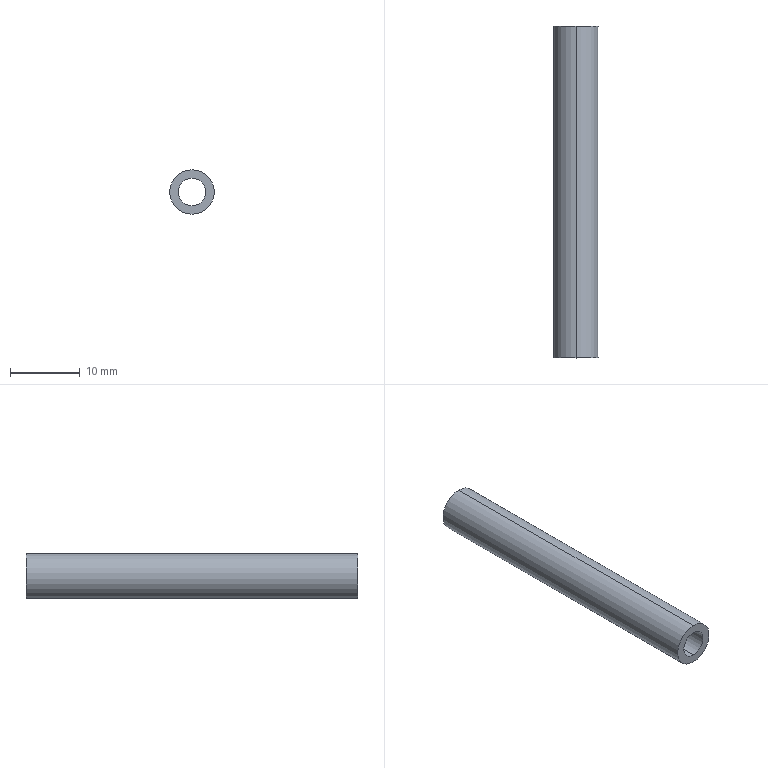Part | NX | features BREP 1 | 1 solid | 6 faces | box 6.35 x 47.5 x 6.35 mm | volume 933.944 mm3 | cylinder 4 | plane 2 | commonest cylinder face diameters 3.91 x2 6.35 x2
STEP:
#1=CARTESIAN_POINT('',(0.,376.,1.955));
#2=VERTEX_POINT('',#1);
#3=CARTESIAN_POINT('',(0.,328.5,1.955));
#4=VERTEX_POINT('',#3);
#5=CARTESIAN_POINT('',(0.,328.5,1.955));
#6=DIRECTION('',(0.,1.,0.));
#7=VECTOR('',#6,1000.);
#8=LINE('',#5,#7);
#9=EDGE_CURVE('',#2,#4,#8,.F.);
#10=ORIENTED_EDGE('',*,*,#9,.T.);
#11=CARTESIAN_POINT('',(0.,328.5,-1.955));
#12=VERTEX_POINT('',#11);
#13=CARTESIAN_POINT('',(0.,328.5,0.));
#14=DIRECTION('',(0.,1.,0.));
#15=DIRECTION('',(-1.,0.,0.));
#16=AXIS2_PLACEMENT_3D('',#13,#14,#15);
#17=CIRCLE('',#16,1.955);
#18=EDGE_CURVE('',#12,#4,#17,.T.);
#19=ORIENTED_EDGE('',*,*,#18,.F.);
#20=CARTESIAN_POINT('',(0.,376.,-1.955));
#21=VERTEX_POINT('',#20);
#22=CARTESIAN_POINT('',(0.,328.5,-1.955));
#23=DIRECTION('',(0.,1.,0.));
#24=VECTOR('',#23,1000.);
#25=LINE('',#22,#24);
#26=EDGE_CURVE('',#21,#12,#25,.F.);
#27=ORIENTED_EDGE('',*,*,#26,.F.);
#28=CARTESIAN_POINT('',(0.,376.,0.));
#29=DIRECTION('',(0.,-1.,0.));
#30=DIRECTION('',(0.,0.,1.));
#31=AXIS2_PLACEMENT_3D('',#28,#29,#30);
#32=CIRCLE('',#31,1.955);
#33=EDGE_CURVE('',#2,#21,#32,.T.);
#34=ORIENTED_EDGE('',*,*,#33,.F.);
#35=EDGE_LOOP('',(#10,#19,#27,#34));
#36=FACE_BOUND('',#35,.T.);
#37=CARTESIAN_POINT('',(0.,376.,0.));
#38=DIRECTION('',(0.,-1.,0.));
#39=DIRECTION('',(0.,0.,-1.));
#40=AXIS2_PLACEMENT_3D('',#37,#38,#39);
#41=CYLINDRICAL_SURFACE('',#40,1.955);
#42=ADVANCED_FACE('',(#36),#41,.F.);
#43=CARTESIAN_POINT('',(0.,376.,-3.175));
#44=VERTEX_POINT('',#43);
#45=CARTESIAN_POINT('',(0.,376.,3.175));
#46=VERTEX_POINT('',#45);
#47=CARTESIAN_POINT('',(0.,376.,0.));
#48=DIRECTION('',(0.,1.,0.));
#49=DIRECTION('',(-1.,0.,0.));
#50=AXIS2_PLACEMENT_3D('',#47,#48,#49);
#51=CIRCLE('',#50,3.175);
#52=EDGE_CURVE('',#44,#46,#51,.T.);
#53=ORIENTED_EDGE('',*,*,#52,.T.);
#54=CARTESIAN_POINT('',(0.,376.,0.));
#55=DIRECTION('',(0.,1.,0.));
#56=DIRECTION('',(0.,0.,1.));
#57=AXIS2_PLACEMENT_3D('',#54,#55,#56);
#58=CIRCLE('',#57,3.175);
#59=EDGE_CURVE('',#46,#44,#58,.T.);
#60=ORIENTED_EDGE('',*,*,#59,.T.);
#61=EDGE_LOOP('',(#53,#60));
#62=FACE_BOUND('',#61,.T.);
#63=CARTESIAN_POINT('',(0.,376.,0.));
#64=DIRECTION('',(0.,-1.,0.));
#65=DIRECTION('',(0.,0.,-1.));
#66=AXIS2_PLACEMENT_3D('',#63,#64,#65);
#67=CIRCLE('',#66,1.955);
#68=EDGE_CURVE('',#21,#2,#67,.T.);
#69=ORIENTED_EDGE('',*,*,#68,.T.);
#70=ORIENTED_EDGE('',*,*,#33,.T.);
#71=EDGE_LOOP('',(#69,#70));
#72=FACE_BOUND('',#71,.T.);
#73=CARTESIAN_POINT('',(0.,376.,0.));
#74=DIRECTION('',(0.,1.,0.));
#75=DIRECTION('',(1.,0.,0.));
#76=AXIS2_PLACEMENT_3D('',#73,#74,#75);
#77=PLANE('',#76);
#78=ADVANCED_FACE('',(#62,#72),#77,.T.);
#79=ORIENTED_EDGE('',*,*,#52,.F.);
#80=CARTESIAN_POINT('',(0.,328.5,-3.175));
#81=VERTEX_POINT('',#80);
#82=CARTESIAN_POINT('',(0.,328.5,-3.175));
#83=DIRECTION('',(0.,1.,0.));
#84=VECTOR('',#83,1000.);
#85=LINE('',#82,#84);
#86=EDGE_CURVE('',#81,#44,#85,.T.);
#87=ORIENTED_EDGE('',*,*,#86,.F.);
#88=CARTESIAN_POINT('',(0.,328.5,3.175));
#89=VERTEX_POINT('',#88);
#90=CARTESIAN_POINT('',(0.,328.5,0.));
#91=DIRECTION('',(0.,-1.,0.));
#92=DIRECTION('',(0.,0.,1.));
#93=AXIS2_PLACEMENT_3D('',#90,#91,#92);
#94=CIRCLE('',#93,3.175);
#95=EDGE_CURVE('',#89,#81,#94,.T.);
#96=ORIENTED_EDGE('',*,*,#95,.F.);
#97=CARTESIAN_POINT('',(0.,328.5,3.175));
#98=DIRECTION('',(0.,1.,0.));
#99=VECTOR('',#98,1000.);
#100=LINE('',#97,#99);
#101=EDGE_CURVE('',#89,#46,#100,.T.);
#102=ORIENTED_EDGE('',*,*,#101,.T.);
#103=EDGE_LOOP('',(#79,#87,#96,#102));
#104=FACE_BOUND('',#103,.T.);
#105=CARTESIAN_POINT('',(0.,376.,0.));
#106=DIRECTION('',(0.,-1.,0.));
#107=DIRECTION('',(0.,0.,-1.));
#108=AXIS2_PLACEMENT_3D('',#105,#106,#107);
#109=CYLINDRICAL_SURFACE('',#108,3.175);
#110=ADVANCED_FACE('',(#104),#109,.T.);
#111=ORIENTED_EDGE('',*,*,#101,.F.);
#112=CARTESIAN_POINT('',(0.,328.5,0.));
#113=DIRECTION('',(0.,-1.,0.));
#114=DIRECTION('',(0.,0.,-1.));
#115=AXIS2_PLACEMENT_3D('',#112,#113,#114);
#116=CIRCLE('',#115,3.175);
#117=EDGE_CURVE('',#81,#89,#116,.T.);
#118=ORIENTED_EDGE('',*,*,#117,.F.);
#119=ORIENTED_EDGE('',*,*,#86,.T.);
#120=ORIENTED_EDGE('',*,*,#59,.F.);
#121=EDGE_LOOP('',(#111,#118,#119,#120));
#122=FACE_BOUND('',#121,.T.);
#123=CARTESIAN_POINT('',(0.,376.,0.));
#124=DIRECTION('',(0.,-1.,0.));
#125=DIRECTION('',(0.,0.,-1.));
#126=AXIS2_PLACEMENT_3D('',#123,#124,#125);
#127=CYLINDRICAL_SURFACE('',#126,3.175);
#128=ADVANCED_FACE('',(#122),#127,.T.);
#129=ORIENTED_EDGE('',*,*,#117,.T.);
#130=ORIENTED_EDGE('',*,*,#95,.T.);
#131=EDGE_LOOP('',(#129,#130));
#132=FACE_BOUND('',#131,.T.);
#133=ORIENTED_EDGE('',*,*,#18,.T.);
#134=CARTESIAN_POINT('',(0.,328.5,0.));
#135=DIRECTION('',(0.,1.,0.));
#136=DIRECTION('',(0.,0.,1.));
#137=AXIS2_PLACEMENT_3D('',#134,#135,#136);
#138=CIRCLE('',#137,1.955);
#139=EDGE_CURVE('',#4,#12,#138,.T.);
#140=ORIENTED_EDGE('',*,*,#139,.T.);
#141=EDGE_LOOP('',(#133,#140));
#142=FACE_BOUND('',#141,.T.);
#143=CARTESIAN_POINT('',(0.,328.5,0.));
#144=DIRECTION('',(0.,1.,0.));
#145=DIRECTION('',(1.,0.,0.));
#146=AXIS2_PLACEMENT_3D('',#143,#144,#145);
#147=PLANE('',#146);
#148=ADVANCED_FACE('',(#132,#142),#147,.F.);
#149=ORIENTED_EDGE('',*,*,#68,.F.);
#150=ORIENTED_EDGE('',*,*,#26,.T.);
#151=ORIENTED_EDGE('',*,*,#139,.F.);
#152=ORIENTED_EDGE('',*,*,#9,.F.);
#153=EDGE_LOOP('',(#149,#150,#151,#152));
#154=FACE_BOUND('',#153,.T.);
#155=CARTESIAN_POINT('',(0.,376.,0.));
#156=DIRECTION('',(0.,-1.,0.));
#157=DIRECTION('',(0.,0.,-1.));
#158=AXIS2_PLACEMENT_3D('',#155,#156,#157);
#159=CYLINDRICAL_SURFACE('',#158,1.955);
#160=ADVANCED_FACE('',(#154),#159,.F.);
#161=CLOSED_SHELL('',(#42,#78,#110,#128,#148,#160));
#162=MANIFOLD_SOLID_BREP('',#161);
#163=(LENGTH_UNIT()NAMED_UNIT(*)SI_UNIT(.MILLI.,.METRE.));
#164=UNCERTAINTY_MEASURE_WITH_UNIT(LENGTH_MEASURE(0.00001),#163,'','');
#165=(NAMED_UNIT(*)PLANE_ANGLE_UNIT()SI_UNIT($,.RADIAN.));
#166=(NAMED_UNIT(*)SI_UNIT($,.STERADIAN.)SOLID_ANGLE_UNIT());
#167=(GEOMETRIC_REPRESENTATION_CONTEXT(3)GLOBAL_UNCERTAINTY_ASSIGNED_CONTEXT((#164))GLOBAL_UNIT_ASSIGNED_CONTEXT((#163,#165,#166))REPRESENTATION_CONTEXT('',''));
#168=ADVANCED_BREP_SHAPE_REPRESENTATION('',(#162),#167);